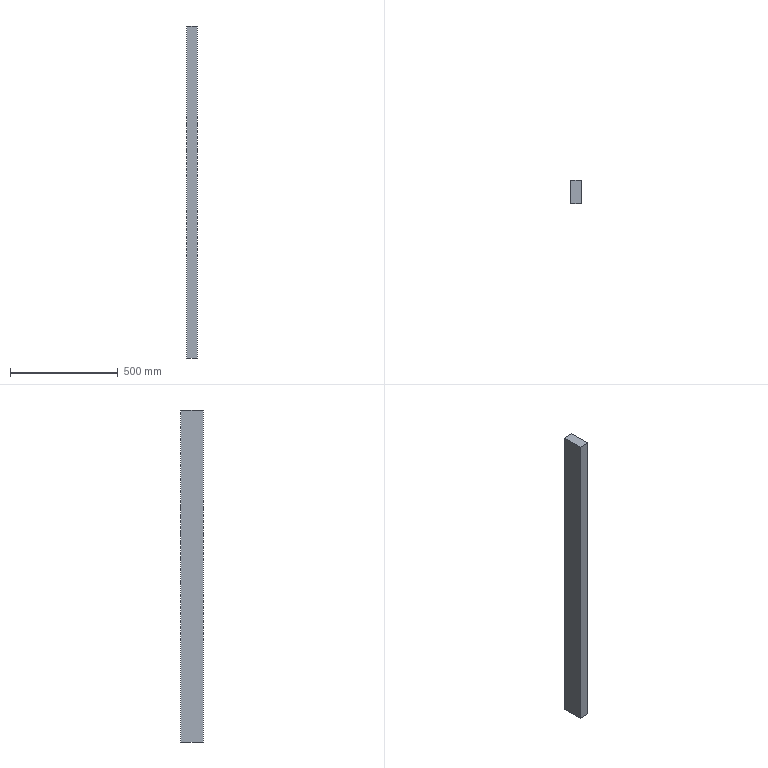Part | SolidWorks | features BaseBody 1 | 1 solid | 74 faces | box 50 x 105 x 1540 mm | volume 8068143 mm3 | cylinder 34 | cone 34 | plane 6 | commonest cylinder face diameters 5 x34